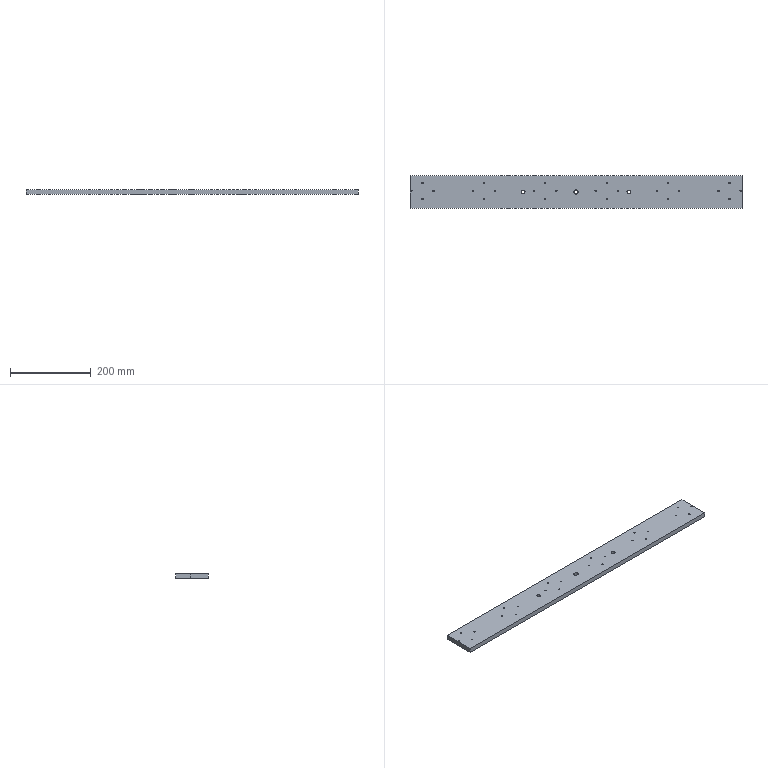Part | SolidWorks | features BaseBody 1 | 1 solid | 66 faces | box 824 x 80 x 12 mm | volume 783419 mm3 | cylinder 58 | plane 8 | commonest cylinder face diameters 3.3 x48 9 x4 30.1 x4 10.5 x2